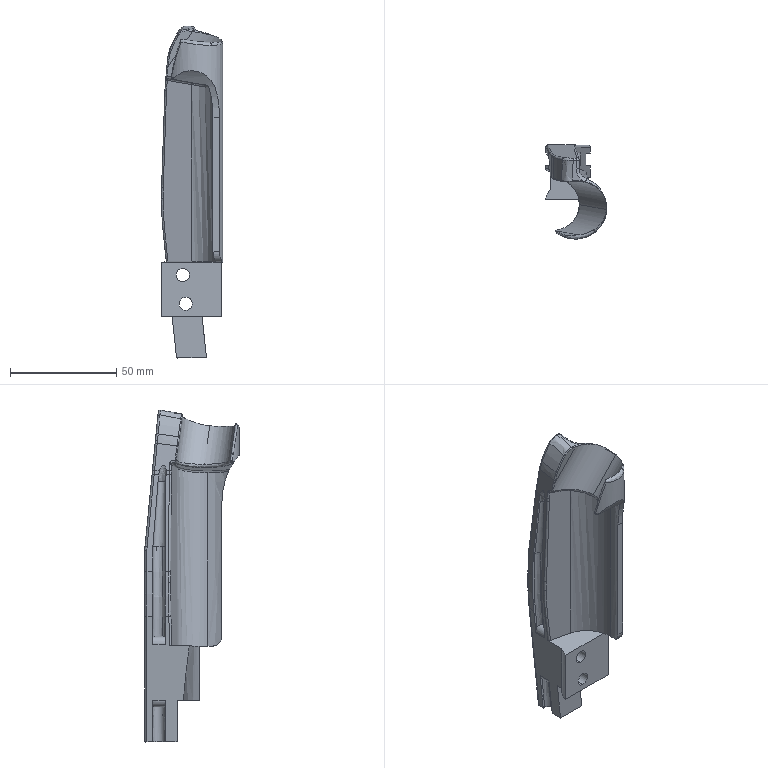Part | STEP file | 101000007584 | 1 solid | 155 faces | box 28.845 x 44.401 x 156.082 mm | volume 37459 mm3 | spline 70 | cylinder 48 | plane 33 | cone 4 | commonest cylinder face diameters 2 x15 1 x5 6.2 x4 7 x4 11 x4 300 x4